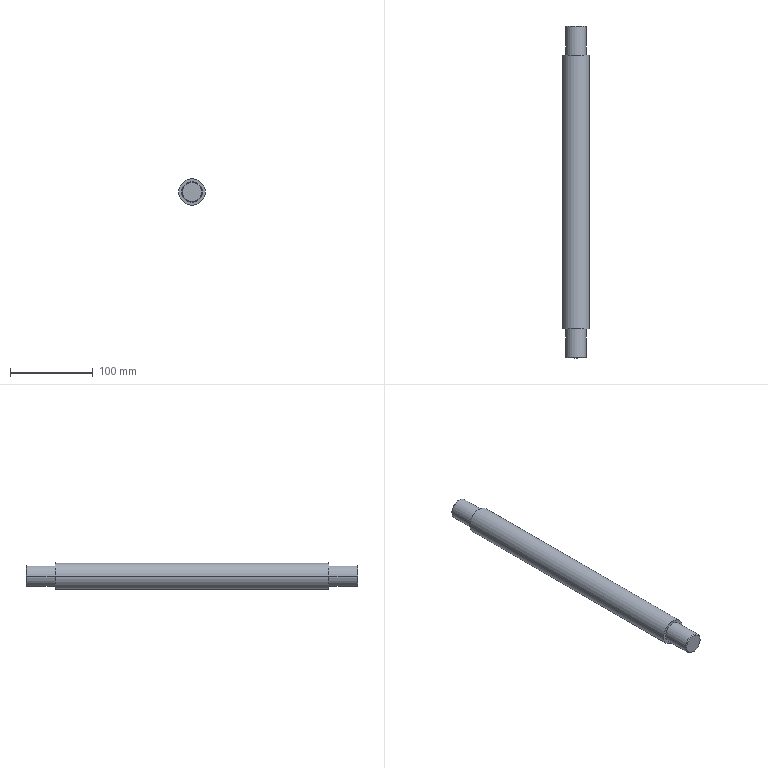Part | SolidWorks | features Chamfer 1, Revolution 1 | 1 solid | 14 faces | box 32 x 400 x 32 mm | volume 299686 mm3 | cylinder 6 | cone 4 | plane 4 | commonest cylinder face diameters 25 x4 32 x2
STEP:
#1=CARTESIAN_POINT('',(-11.5,400.,0.));
#2=VERTEX_POINT('',#1);
#3=CARTESIAN_POINT('',(11.5,400.,0.));
#4=VERTEX_POINT('',#3);
#5=CARTESIAN_POINT('',(0.,400.,0.));
#6=DIRECTION('',(0.,1.,0.));
#7=DIRECTION('',(1.,0.,0.));
#8=AXIS2_PLACEMENT_3D('',#5,#6,#7);
#9=CIRCLE('',#8,11.5);
#10=EDGE_CURVE('',#2,#4,#9,.T.);
#11=ORIENTED_EDGE('',*,*,#10,.F.);
#12=CARTESIAN_POINT('',(-12.5,399.,0.));
#13=VERTEX_POINT('',#12);
#14=CARTESIAN_POINT('',(-11.5,400.,0.));
#15=DIRECTION('',(-0.7071,-0.7071,0.));
#16=VECTOR('',#15,1000.);
#17=LINE('',#14,#16);
#18=EDGE_CURVE('',#2,#13,#17,.T.);
#19=ORIENTED_EDGE('',*,*,#18,.T.);
#20=CARTESIAN_POINT('',(12.5,399.,0.));
#21=VERTEX_POINT('',#20);
#22=CARTESIAN_POINT('',(0.,399.,0.));
#23=DIRECTION('',(0.,-1.,0.));
#24=DIRECTION('',(1.,0.,0.));
#25=AXIS2_PLACEMENT_3D('',#22,#23,#24);
#26=CIRCLE('',#25,12.5);
#27=EDGE_CURVE('',#21,#13,#26,.T.);
#28=ORIENTED_EDGE('',*,*,#27,.F.);
#29=CARTESIAN_POINT('',(11.5,400.,0.));
#30=DIRECTION('',(0.7071,-0.7071,0.));
#31=VECTOR('',#30,1000.);
#32=LINE('',#29,#31);
#33=EDGE_CURVE('',#4,#21,#32,.T.);
#34=ORIENTED_EDGE('',*,*,#33,.F.);
#35=EDGE_LOOP('',(#11,#19,#28,#34));
#36=FACE_OUTER_BOUND('',#35,.T.);
#37=CARTESIAN_POINT('',(0.,400.,0.));
#38=DIRECTION('',(0.,-1.,0.));
#39=DIRECTION('',(1.,0.,0.));
#40=AXIS2_PLACEMENT_3D('',#37,#38,#39);
#41=CONICAL_SURFACE('',#40,11.5,0.7854);
#42=ADVANCED_FACE('',(#36),#41,.T.);
#43=CARTESIAN_POINT('',(11.5,0.,0.));
#44=VERTEX_POINT('',#43);
#45=CARTESIAN_POINT('',(-11.5,0.,0.));
#46=VERTEX_POINT('',#45);
#47=CARTESIAN_POINT('',(0.,0.,0.));
#48=DIRECTION('',(0.,-1.,0.));
#49=DIRECTION('',(-1.,0.,0.));
#50=AXIS2_PLACEMENT_3D('',#47,#48,#49);
#51=CIRCLE('',#50,11.5);
#52=EDGE_CURVE('',#44,#46,#51,.T.);
#53=ORIENTED_EDGE('',*,*,#52,.F.);
#54=CARTESIAN_POINT('',(12.5,1.,0.));
#55=VERTEX_POINT('',#54);
#56=CARTESIAN_POINT('',(12.5,1.,0.));
#57=DIRECTION('',(0.7071,0.7071,0.));
#58=VECTOR('',#57,1000.);
#59=LINE('',#56,#58);
#60=EDGE_CURVE('',#44,#55,#59,.T.);
#61=ORIENTED_EDGE('',*,*,#60,.T.);
#62=CARTESIAN_POINT('',(-12.5,1.,0.));
#63=VERTEX_POINT('',#62);
#64=CARTESIAN_POINT('',(0.,1.,0.));
#65=DIRECTION('',(0.,1.,0.));
#66=DIRECTION('',(-1.,0.,0.));
#67=AXIS2_PLACEMENT_3D('',#64,#65,#66);
#68=CIRCLE('',#67,12.5);
#69=EDGE_CURVE('',#63,#55,#68,.T.);
#70=ORIENTED_EDGE('',*,*,#69,.F.);
#71=CARTESIAN_POINT('',(-12.5,1.,0.));
#72=DIRECTION('',(-0.7071,0.7071,0.));
#73=VECTOR('',#72,1000.);
#74=LINE('',#71,#73);
#75=EDGE_CURVE('',#46,#63,#74,.T.);
#76=ORIENTED_EDGE('',*,*,#75,.F.);
#77=EDGE_LOOP('',(#53,#61,#70,#76));
#78=FACE_OUTER_BOUND('',#77,.T.);
#79=CARTESIAN_POINT('',(0.,1.,0.));
#80=DIRECTION('',(0.,1.,0.));
#81=DIRECTION('',(-1.,0.,0.));
#82=AXIS2_PLACEMENT_3D('',#79,#80,#81);
#83=CONICAL_SURFACE('',#82,12.5,0.7854);
#84=ADVANCED_FACE('',(#78),#83,.T.);
#85=CARTESIAN_POINT('',(-12.5,365.,0.));
#86=VERTEX_POINT('',#85);
#87=CARTESIAN_POINT('',(12.5,365.,0.));
#88=VERTEX_POINT('',#87);
#89=CARTESIAN_POINT('',(0.,365.,0.));
#90=DIRECTION('',(0.,1.,0.));
#91=DIRECTION('',(-1.,0.,0.));
#92=AXIS2_PLACEMENT_3D('',#89,#90,#91);
#93=CIRCLE('',#92,12.5);
#94=EDGE_CURVE('',#86,#88,#93,.T.);
#95=ORIENTED_EDGE('',*,*,#94,.T.);
#96=CARTESIAN_POINT('',(12.5,400.,0.));
#97=DIRECTION('',(0.,1.,0.));
#98=VECTOR('',#97,1000.);
#99=LINE('',#96,#98);
#100=EDGE_CURVE('',#88,#21,#99,.T.);
#101=ORIENTED_EDGE('',*,*,#100,.T.);
#102=ORIENTED_EDGE('',*,*,#27,.T.);
#103=CARTESIAN_POINT('',(-12.5,400.,0.));
#104=DIRECTION('',(0.,1.,0.));
#105=VECTOR('',#104,1000.);
#106=LINE('',#103,#105);
#107=EDGE_CURVE('',#86,#13,#106,.T.);
#108=ORIENTED_EDGE('',*,*,#107,.F.);
#109=EDGE_LOOP('',(#95,#101,#102,#108));
#110=FACE_OUTER_BOUND('',#109,.T.);
#111=CARTESIAN_POINT('',(0.,400.,0.));
#112=DIRECTION('',(0.,1.,0.));
#113=DIRECTION('',(-1.,0.,0.));
#114=AXIS2_PLACEMENT_3D('',#111,#112,#113);
#115=CYLINDRICAL_SURFACE('',#114,12.5);
#116=ADVANCED_FACE('',(#110),#115,.T.);
#117=CARTESIAN_POINT('',(-16.,35.,0.));
#118=VERTEX_POINT('',#117);
#119=CARTESIAN_POINT('',(16.,35.,0.));
#120=VERTEX_POINT('',#119);
#121=CARTESIAN_POINT('',(0.,35.,0.));
#122=DIRECTION('',(0.,1.,0.));
#123=DIRECTION('',(-1.,0.,0.));
#124=AXIS2_PLACEMENT_3D('',#121,#122,#123);
#125=CIRCLE('',#124,16.);
#126=EDGE_CURVE('',#118,#120,#125,.T.);
#127=ORIENTED_EDGE('',*,*,#126,.T.);
#128=CARTESIAN_POINT('',(16.,365.,0.));
#129=VERTEX_POINT('',#128);
#130=CARTESIAN_POINT('',(16.,400.,0.));
#131=DIRECTION('',(0.,1.,0.));
#132=VECTOR('',#131,1000.);
#133=LINE('',#130,#132);
#134=EDGE_CURVE('',#120,#129,#133,.T.);
#135=ORIENTED_EDGE('',*,*,#134,.T.);
#136=CARTESIAN_POINT('',(-16.,365.,0.));
#137=VERTEX_POINT('',#136);
#138=CARTESIAN_POINT('',(0.,365.,0.));
#139=DIRECTION('',(0.,1.,0.));
#140=DIRECTION('',(-1.,0.,0.));
#141=AXIS2_PLACEMENT_3D('',#138,#139,#140);
#142=CIRCLE('',#141,16.);
#143=EDGE_CURVE('',#137,#129,#142,.T.);
#144=ORIENTED_EDGE('',*,*,#143,.F.);
#145=CARTESIAN_POINT('',(-16.,400.,0.));
#146=DIRECTION('',(0.,1.,0.));
#147=VECTOR('',#146,1000.);
#148=LINE('',#145,#147);
#149=EDGE_CURVE('',#118,#137,#148,.T.);
#150=ORIENTED_EDGE('',*,*,#149,.F.);
#151=EDGE_LOOP('',(#127,#135,#144,#150));
#152=FACE_OUTER_BOUND('',#151,.T.);
#153=CARTESIAN_POINT('',(0.,400.,0.));
#154=DIRECTION('',(0.,1.,0.));
#155=DIRECTION('',(-1.,0.,0.));
#156=AXIS2_PLACEMENT_3D('',#153,#154,#155);
#157=CYLINDRICAL_SURFACE('',#156,16.);
#158=ADVANCED_FACE('',(#152),#157,.T.);
#159=ORIENTED_EDGE('',*,*,#69,.T.);
#160=CARTESIAN_POINT('',(12.5,35.,0.));
#161=VERTEX_POINT('',#160);
#162=CARTESIAN_POINT('',(12.5,400.,0.));
#163=DIRECTION('',(0.,1.,0.));
#164=VECTOR('',#163,1000.);
#165=LINE('',#162,#164);
#166=EDGE_CURVE('',#55,#161,#165,.T.);
#167=ORIENTED_EDGE('',*,*,#166,.T.);
#168=CARTESIAN_POINT('',(-12.5,35.,0.));
#169=VERTEX_POINT('',#168);
#170=CARTESIAN_POINT('',(0.,35.,0.));
#171=DIRECTION('',(0.,1.,0.));
#172=DIRECTION('',(-1.,0.,0.));
#173=AXIS2_PLACEMENT_3D('',#170,#171,#172);
#174=CIRCLE('',#173,12.5);
#175=EDGE_CURVE('',#169,#161,#174,.T.);
#176=ORIENTED_EDGE('',*,*,#175,.F.);
#177=CARTESIAN_POINT('',(-12.5,400.,0.));
#178=DIRECTION('',(0.,1.,0.));
#179=VECTOR('',#178,1000.);
#180=LINE('',#177,#179);
#181=EDGE_CURVE('',#63,#169,#180,.T.);
#182=ORIENTED_EDGE('',*,*,#181,.F.);
#183=EDGE_LOOP('',(#159,#167,#176,#182));
#184=FACE_OUTER_BOUND('',#183,.T.);
#185=CARTESIAN_POINT('',(0.,400.,0.));
#186=DIRECTION('',(0.,1.,0.));
#187=DIRECTION('',(-1.,0.,0.));
#188=AXIS2_PLACEMENT_3D('',#185,#186,#187);
#189=CYLINDRICAL_SURFACE('',#188,12.5);
#190=ADVANCED_FACE('',(#184),#189,.T.);
#191=CARTESIAN_POINT('',(0.,0.,0.));
#192=DIRECTION('',(0.,-1.,0.));
#193=DIRECTION('',(-1.,0.,0.));
#194=AXIS2_PLACEMENT_3D('',#191,#192,#193);
#195=CIRCLE('',#194,11.5);
#196=EDGE_CURVE('',#46,#44,#195,.T.);
#197=ORIENTED_EDGE('',*,*,#196,.T.);
#198=ORIENTED_EDGE('',*,*,#52,.T.);
#199=EDGE_LOOP('',(#197,#198));
#200=FACE_OUTER_BOUND('',#199,.T.);
#201=CARTESIAN_POINT('',(0.,0.,0.));
#202=DIRECTION('',(0.,1.,0.));
#203=DIRECTION('',(-1.,0.,0.));
#204=AXIS2_PLACEMENT_3D('',#201,#202,#203);
#205=PLANE('',#204);
#206=ADVANCED_FACE('',(#200),#205,.F.);
#207=ORIENTED_EDGE('',*,*,#166,.F.);
#208=CARTESIAN_POINT('',(0.,1.,0.));
#209=DIRECTION('',(0.,1.,0.));
#210=DIRECTION('',(-1.,0.,0.));
#211=AXIS2_PLACEMENT_3D('',#208,#209,#210);
#212=CIRCLE('',#211,12.5);
#213=EDGE_CURVE('',#55,#63,#212,.T.);
#214=ORIENTED_EDGE('',*,*,#213,.T.);
#215=ORIENTED_EDGE('',*,*,#181,.T.);
#216=CARTESIAN_POINT('',(0.,35.,0.));
#217=DIRECTION('',(0.,1.,0.));
#218=DIRECTION('',(-1.,0.,0.));
#219=AXIS2_PLACEMENT_3D('',#216,#217,#218);
#220=CIRCLE('',#219,12.5);
#221=EDGE_CURVE('',#161,#169,#220,.T.);
#222=ORIENTED_EDGE('',*,*,#221,.F.);
#223=EDGE_LOOP('',(#207,#214,#215,#222));
#224=FACE_OUTER_BOUND('',#223,.T.);
#225=CARTESIAN_POINT('',(0.,400.,0.));
#226=DIRECTION('',(0.,1.,0.));
#227=DIRECTION('',(-1.,0.,0.));
#228=AXIS2_PLACEMENT_3D('',#225,#226,#227);
#229=CYLINDRICAL_SURFACE('',#228,12.5);
#230=ADVANCED_FACE('',(#224),#229,.T.);
#231=ORIENTED_EDGE('',*,*,#126,.F.);
#232=CARTESIAN_POINT('',(0.,35.,0.));
#233=DIRECTION('',(0.,1.,0.));
#234=DIRECTION('',(-1.,0.,0.));
#235=AXIS2_PLACEMENT_3D('',#232,#233,#234);
#236=CIRCLE('',#235,16.);
#237=EDGE_CURVE('',#120,#118,#236,.T.);
#238=ORIENTED_EDGE('',*,*,#237,.F.);
#239=EDGE_LOOP('',(#231,#238));
#240=FACE_OUTER_BOUND('',#239,.T.);
#241=ORIENTED_EDGE('',*,*,#175,.T.);
#242=ORIENTED_EDGE('',*,*,#221,.T.);
#243=EDGE_LOOP('',(#241,#242));
#244=FACE_BOUND('',#243,.T.);
#245=CARTESIAN_POINT('',(12.5,35.,0.));
#246=DIRECTION('',(0.,1.,0.));
#247=DIRECTION('',(-1.,0.,0.));
#248=AXIS2_PLACEMENT_3D('',#245,#246,#247);
#249=PLANE('',#248);
#250=ADVANCED_FACE('',(#240,#244),#249,.F.);
#251=ORIENTED_EDGE('',*,*,#134,.F.);
#252=ORIENTED_EDGE('',*,*,#237,.T.);
#253=ORIENTED_EDGE('',*,*,#149,.T.);
#254=CARTESIAN_POINT('',(0.,365.,0.));
#255=DIRECTION('',(0.,1.,0.));
#256=DIRECTION('',(-1.,0.,0.));
#257=AXIS2_PLACEMENT_3D('',#254,#255,#256);
#258=CIRCLE('',#257,16.);
#259=EDGE_CURVE('',#129,#137,#258,.T.);
#260=ORIENTED_EDGE('',*,*,#259,.F.);
#261=EDGE_LOOP('',(#251,#252,#253,#260));
#262=FACE_OUTER_BOUND('',#261,.T.);
#263=CARTESIAN_POINT('',(0.,400.,0.));
#264=DIRECTION('',(0.,1.,0.));
#265=DIRECTION('',(-1.,0.,0.));
#266=AXIS2_PLACEMENT_3D('',#263,#264,#265);
#267=CYLINDRICAL_SURFACE('',#266,16.);
#268=ADVANCED_FACE('',(#262),#267,.T.);
#269=ORIENTED_EDGE('',*,*,#94,.F.);
#270=CARTESIAN_POINT('',(0.,365.,0.));
#271=DIRECTION('',(0.,1.,0.));
#272=DIRECTION('',(-1.,0.,0.));
#273=AXIS2_PLACEMENT_3D('',#270,#271,#272);
#274=CIRCLE('',#273,12.5);
#275=EDGE_CURVE('',#88,#86,#274,.T.);
#276=ORIENTED_EDGE('',*,*,#275,.F.);
#277=EDGE_LOOP('',(#269,#276));
#278=FACE_BOUND('',#277,.T.);
#279=ORIENTED_EDGE('',*,*,#143,.T.);
#280=ORIENTED_EDGE('',*,*,#259,.T.);
#281=EDGE_LOOP('',(#279,#280));
#282=FACE_OUTER_BOUND('',#281,.T.);
#283=CARTESIAN_POINT('',(16.,365.,0.));
#284=DIRECTION('',(0.,-1.,0.));
#285=DIRECTION('',(1.,0.,0.));
#286=AXIS2_PLACEMENT_3D('',#283,#284,#285);
#287=PLANE('',#286);
#288=ADVANCED_FACE('',(#278,#282),#287,.F.);
#289=ORIENTED_EDGE('',*,*,#100,.F.);
#290=ORIENTED_EDGE('',*,*,#275,.T.);
#291=ORIENTED_EDGE('',*,*,#107,.T.);
#292=CARTESIAN_POINT('',(0.,399.,0.));
#293=DIRECTION('',(0.,-1.,0.));
#294=DIRECTION('',(1.,0.,0.));
#295=AXIS2_PLACEMENT_3D('',#292,#293,#294);
#296=CIRCLE('',#295,12.5);
#297=EDGE_CURVE('',#13,#21,#296,.T.);
#298=ORIENTED_EDGE('',*,*,#297,.T.);
#299=EDGE_LOOP('',(#289,#290,#291,#298));
#300=FACE_OUTER_BOUND('',#299,.T.);
#301=CARTESIAN_POINT('',(0.,400.,0.));
#302=DIRECTION('',(0.,1.,0.));
#303=DIRECTION('',(-1.,0.,0.));
#304=AXIS2_PLACEMENT_3D('',#301,#302,#303);
#305=CYLINDRICAL_SURFACE('',#304,12.5);
#306=ADVANCED_FACE('',(#300),#305,.T.);
#307=CARTESIAN_POINT('',(0.,400.,0.));
#308=DIRECTION('',(0.,1.,0.));
#309=DIRECTION('',(1.,0.,0.));
#310=AXIS2_PLACEMENT_3D('',#307,#308,#309);
#311=CIRCLE('',#310,11.5);
#312=EDGE_CURVE('',#4,#2,#311,.T.);
#313=ORIENTED_EDGE('',*,*,#312,.T.);
#314=ORIENTED_EDGE('',*,*,#10,.T.);
#315=EDGE_LOOP('',(#313,#314));
#316=FACE_OUTER_BOUND('',#315,.T.);
#317=CARTESIAN_POINT('',(12.5,400.,0.));
#318=DIRECTION('',(0.,-1.,0.));
#319=DIRECTION('',(1.,0.,0.));
#320=AXIS2_PLACEMENT_3D('',#317,#318,#319);
#321=PLANE('',#320);
#322=ADVANCED_FACE('',(#316),#321,.F.);
#323=ORIENTED_EDGE('',*,*,#60,.F.);
#324=ORIENTED_EDGE('',*,*,#196,.F.);
#325=ORIENTED_EDGE('',*,*,#75,.T.);
#326=ORIENTED_EDGE('',*,*,#213,.F.);
#327=EDGE_LOOP('',(#323,#324,#325,#326));
#328=FACE_OUTER_BOUND('',#327,.T.);
#329=CARTESIAN_POINT('',(0.,1.,0.));
#330=DIRECTION('',(0.,1.,0.));
#331=DIRECTION('',(-1.,0.,0.));
#332=AXIS2_PLACEMENT_3D('',#329,#330,#331);
#333=CONICAL_SURFACE('',#332,12.5,0.7854);
#334=ADVANCED_FACE('',(#328),#333,.T.);
#335=ORIENTED_EDGE('',*,*,#18,.F.);
#336=ORIENTED_EDGE('',*,*,#312,.F.);
#337=ORIENTED_EDGE('',*,*,#33,.T.);
#338=ORIENTED_EDGE('',*,*,#297,.F.);
#339=EDGE_LOOP('',(#335,#336,#337,#338));
#340=FACE_OUTER_BOUND('',#339,.T.);
#341=CARTESIAN_POINT('',(0.,400.,0.));
#342=DIRECTION('',(0.,-1.,0.));
#343=DIRECTION('',(1.,0.,0.));
#344=AXIS2_PLACEMENT_3D('',#341,#342,#343);
#345=CONICAL_SURFACE('',#344,11.5,0.7854);
#346=ADVANCED_FACE('',(#340),#345,.T.);
#347=CLOSED_SHELL('',(#42,#84,#116,#158,#190,#206,#230,#250,#268,#288,#306,#322,#334,#346));
#348=MANIFOLD_SOLID_BREP('',#347);
#349=CARTESIAN_POINT('',(0.,0.,0.));
#350=DIRECTION('',(0.,0.,1.));
#351=DIRECTION('',(1.,0.,0.));
#352=AXIS2_PLACEMENT_3D('',#349,#350,#351);
#353=(LENGTH_UNIT()NAMED_UNIT(*)SI_UNIT(.MILLI.,.METRE.));
#354=UNCERTAINTY_MEASURE_WITH_UNIT(LENGTH_MEASURE(0.00001),#353,'','');
#355=(NAMED_UNIT(*)PLANE_ANGLE_UNIT()SI_UNIT($,.RADIAN.));
#356=(NAMED_UNIT(*)SI_UNIT($,.STERADIAN.)SOLID_ANGLE_UNIT());
#357=(GEOMETRIC_REPRESENTATION_CONTEXT(3)GLOBAL_UNCERTAINTY_ASSIGNED_CONTEXT((#354))GLOBAL_UNIT_ASSIGNED_CONTEXT((#353,#355,#356))REPRESENTATION_CONTEXT('',''));
#358=ADVANCED_BREP_SHAPE_REPRESENTATION('',(#348,#352),#357);